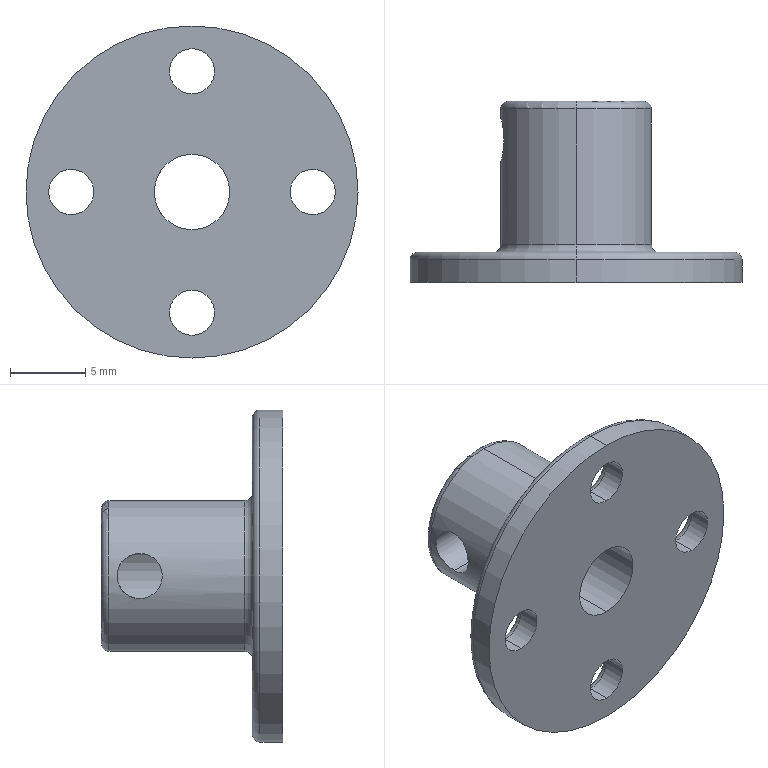Part | STEP file | Flange coupling 5 | 1 solid | 33 faces | box 22 x 12 x 22 mm | volume 1230 mm3 | cylinder 16 | torus 14 | plane 3 | commonest cylinder face diameters 3 x10 5 x2 10 x2 22 x2